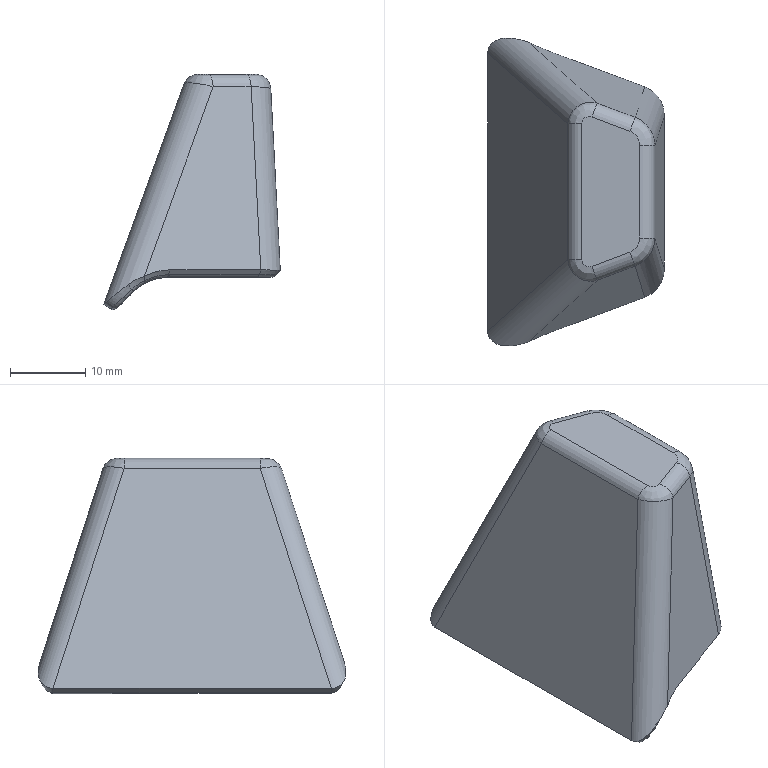Part | SolidWorks | features BaseBody 1 | 1 solid | 147 faces | box 23.497 x 40.981 x 31.302 mm | volume 9658 mm3 | cylinder 53 | plane 36 | spline 34 | sphere 18 | cone 4 | torus 2 | commonest cylinder face diameters 1 x28 2 x9 4 x4 1.893 x2 4.2 x2 6 x2